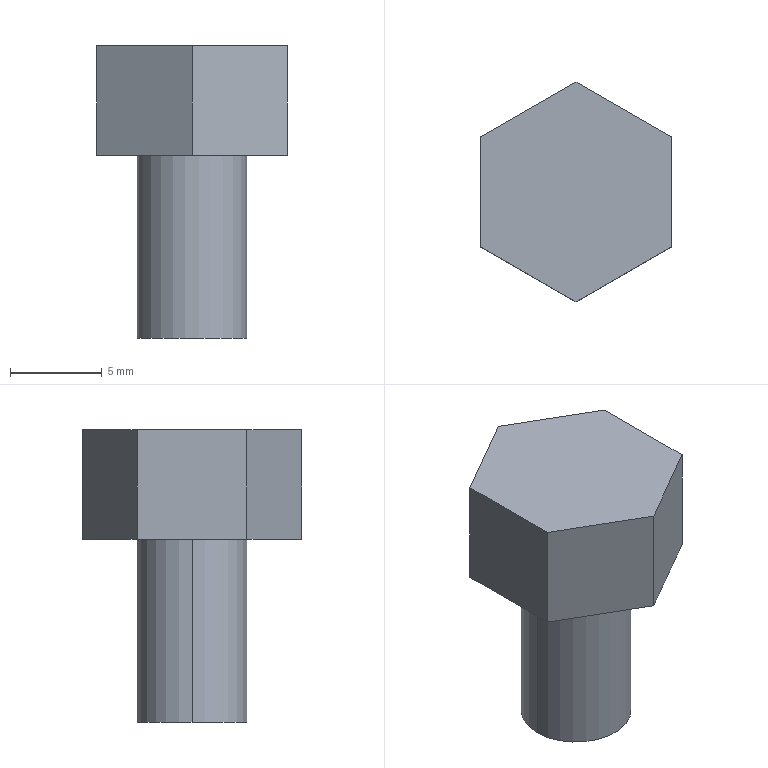Part | SolidWorks | features Extrusion 1, ICE 1 | 1 solid | 11 faces | box 10.392 x 12 x 16 mm | volume 843.928 mm3 | plane 9 | cylinder 2 | commonest cylinder face diameters 6 x2
STEP:
#1=CARTESIAN_POINT('',(3.,0.,10.));
#2=VERTEX_POINT('',#1);
#3=CARTESIAN_POINT('',(-3.,0.,10.));
#4=VERTEX_POINT('',#3);
#5=CARTESIAN_POINT('',(0.,0.,10.));
#6=DIRECTION('',(0.,0.,1.));
#7=DIRECTION('',(1.,0.,0.));
#8=AXIS2_PLACEMENT_3D('',#5,#6,#7);
#9=CIRCLE('',#8,3.);
#10=EDGE_CURVE('',#2,#4,#9,.T.);
#11=ORIENTED_EDGE('',*,*,#10,.F.);
#12=CARTESIAN_POINT('',(3.,0.,0.));
#13=VERTEX_POINT('',#12);
#14=CARTESIAN_POINT('',(3.,0.,10.));
#15=DIRECTION('',(0.,0.,-1.));
#16=VECTOR('',#15,1000.);
#17=LINE('',#14,#16);
#18=EDGE_CURVE('',#2,#13,#17,.T.);
#19=ORIENTED_EDGE('',*,*,#18,.T.);
#20=CARTESIAN_POINT('',(-3.,0.,0.));
#21=VERTEX_POINT('',#20);
#22=CARTESIAN_POINT('',(0.,0.,0.));
#23=DIRECTION('',(0.,0.,1.));
#24=DIRECTION('',(1.,0.,0.));
#25=AXIS2_PLACEMENT_3D('',#22,#23,#24);
#26=CIRCLE('',#25,3.);
#27=EDGE_CURVE('',#13,#21,#26,.T.);
#28=ORIENTED_EDGE('',*,*,#27,.T.);
#29=CARTESIAN_POINT('',(-3.,0.,10.));
#30=DIRECTION('',(0.,0.,-1.));
#31=VECTOR('',#30,1000.);
#32=LINE('',#29,#31);
#33=EDGE_CURVE('',#4,#21,#32,.T.);
#34=ORIENTED_EDGE('',*,*,#33,.F.);
#35=EDGE_LOOP('',(#11,#19,#28,#34));
#36=FACE_OUTER_BOUND('',#35,.T.);
#37=CARTESIAN_POINT('',(0.,0.,10.));
#38=DIRECTION('',(0.,0.,-1.));
#39=DIRECTION('',(-1.,0.,0.));
#40=AXIS2_PLACEMENT_3D('',#37,#38,#39);
#41=CYLINDRICAL_SURFACE('',#40,3.);
#42=ADVANCED_FACE('',(#36),#41,.T.);
#43=ORIENTED_EDGE('',*,*,#18,.F.);
#44=CARTESIAN_POINT('',(0.,0.,10.));
#45=DIRECTION('',(0.,0.,1.));
#46=DIRECTION('',(1.,0.,0.));
#47=AXIS2_PLACEMENT_3D('',#44,#45,#46);
#48=CIRCLE('',#47,3.);
#49=EDGE_CURVE('',#4,#2,#48,.T.);
#50=ORIENTED_EDGE('',*,*,#49,.F.);
#51=ORIENTED_EDGE('',*,*,#33,.T.);
#52=CARTESIAN_POINT('',(0.,0.,0.));
#53=DIRECTION('',(0.,0.,1.));
#54=DIRECTION('',(1.,0.,0.));
#55=AXIS2_PLACEMENT_3D('',#52,#53,#54);
#56=CIRCLE('',#55,3.);
#57=EDGE_CURVE('',#21,#13,#56,.T.);
#58=ORIENTED_EDGE('',*,*,#57,.T.);
#59=EDGE_LOOP('',(#43,#50,#51,#58));
#60=FACE_OUTER_BOUND('',#59,.T.);
#61=CARTESIAN_POINT('',(0.,0.,10.));
#62=DIRECTION('',(0.,0.,-1.));
#63=DIRECTION('',(-1.,0.,0.));
#64=AXIS2_PLACEMENT_3D('',#61,#62,#63);
#65=CYLINDRICAL_SURFACE('',#64,3.);
#66=ADVANCED_FACE('',(#60),#65,.T.);
#67=ORIENTED_EDGE('',*,*,#57,.F.);
#68=ORIENTED_EDGE('',*,*,#27,.F.);
#69=EDGE_LOOP('',(#67,#68));
#70=FACE_OUTER_BOUND('',#69,.T.);
#71=CARTESIAN_POINT('',(0.,0.,0.));
#72=DIRECTION('',(0.,0.,1.));
#73=DIRECTION('',(1.,0.,0.));
#74=AXIS2_PLACEMENT_3D('',#71,#72,#73);
#75=PLANE('',#74);
#76=ADVANCED_FACE('',(#70),#75,.F.);
#77=CARTESIAN_POINT('',(-5.196,3.,10.));
#78=VERTEX_POINT('',#77);
#79=CARTESIAN_POINT('',(-5.196,-3.,10.));
#80=VERTEX_POINT('',#79);
#81=CARTESIAN_POINT('',(-5.196,3.,10.));
#82=DIRECTION('',(0.,-1.,0.));
#83=VECTOR('',#82,1000.);
#84=LINE('',#81,#83);
#85=EDGE_CURVE('',#78,#80,#84,.T.);
#86=ORIENTED_EDGE('',*,*,#85,.T.);
#87=CARTESIAN_POINT('',(-5.196,-3.,16.));
#88=VERTEX_POINT('',#87);
#89=CARTESIAN_POINT('',(-5.196,-3.,16.));
#90=DIRECTION('',(0.,0.,-1.));
#91=VECTOR('',#90,1000.);
#92=LINE('',#89,#91);
#93=EDGE_CURVE('',#88,#80,#92,.T.);
#94=ORIENTED_EDGE('',*,*,#93,.F.);
#95=CARTESIAN_POINT('',(-5.196,3.,16.));
#96=VERTEX_POINT('',#95);
#97=CARTESIAN_POINT('',(-5.196,3.,16.));
#98=DIRECTION('',(0.,-1.,0.));
#99=VECTOR('',#98,1000.);
#100=LINE('',#97,#99);
#101=EDGE_CURVE('',#96,#88,#100,.T.);
#102=ORIENTED_EDGE('',*,*,#101,.F.);
#103=CARTESIAN_POINT('',(-5.196,3.,16.));
#104=DIRECTION('',(0.,0.,-1.));
#105=VECTOR('',#104,1000.);
#106=LINE('',#103,#105);
#107=EDGE_CURVE('',#96,#78,#106,.T.);
#108=ORIENTED_EDGE('',*,*,#107,.T.);
#109=EDGE_LOOP('',(#86,#94,#102,#108));
#110=FACE_OUTER_BOUND('',#109,.T.);
#111=CARTESIAN_POINT('',(-5.196,3.,16.));
#112=DIRECTION('',(1.,0.,0.));
#113=DIRECTION('',(0.,0.,-1.));
#114=AXIS2_PLACEMENT_3D('',#111,#112,#113);
#115=PLANE('',#114);
#116=ADVANCED_FACE('',(#110),#115,.F.);
#117=CARTESIAN_POINT('',(0.,-6.,10.));
#118=VERTEX_POINT('',#117);
#119=CARTESIAN_POINT('',(-5.196,-3.,10.));
#120=DIRECTION('',(0.866,-0.5,0.));
#121=VECTOR('',#120,1000.);
#122=LINE('',#119,#121);
#123=EDGE_CURVE('',#80,#118,#122,.T.);
#124=ORIENTED_EDGE('',*,*,#123,.T.);
#125=CARTESIAN_POINT('',(0.,-6.,16.));
#126=VERTEX_POINT('',#125);
#127=CARTESIAN_POINT('',(0.,-6.,16.));
#128=DIRECTION('',(0.,0.,-1.));
#129=VECTOR('',#128,1000.);
#130=LINE('',#127,#129);
#131=EDGE_CURVE('',#126,#118,#130,.T.);
#132=ORIENTED_EDGE('',*,*,#131,.F.);
#133=CARTESIAN_POINT('',(-5.196,-3.,16.));
#134=DIRECTION('',(0.866,-0.5,0.));
#135=VECTOR('',#134,1000.);
#136=LINE('',#133,#135);
#137=EDGE_CURVE('',#88,#126,#136,.T.);
#138=ORIENTED_EDGE('',*,*,#137,.F.);
#139=ORIENTED_EDGE('',*,*,#93,.T.);
#140=EDGE_LOOP('',(#124,#132,#138,#139));
#141=FACE_OUTER_BOUND('',#140,.T.);
#142=CARTESIAN_POINT('',(-5.196,-3.,16.));
#143=DIRECTION('',(0.5,0.866,0.));
#144=DIRECTION('',(-0.866,0.5,0.));
#145=AXIS2_PLACEMENT_3D('',#142,#143,#144);
#146=PLANE('',#145);
#147=ADVANCED_FACE('',(#141),#146,.F.);
#148=CARTESIAN_POINT('',(5.196,-3.,10.));
#149=VERTEX_POINT('',#148);
#150=CARTESIAN_POINT('',(0.,-6.,10.));
#151=DIRECTION('',(0.866,0.5,0.));
#152=VECTOR('',#151,1000.);
#153=LINE('',#150,#152);
#154=EDGE_CURVE('',#118,#149,#153,.T.);
#155=ORIENTED_EDGE('',*,*,#154,.T.);
#156=CARTESIAN_POINT('',(5.196,-3.,16.));
#157=VERTEX_POINT('',#156);
#158=CARTESIAN_POINT('',(5.196,-3.,16.));
#159=DIRECTION('',(0.,0.,-1.));
#160=VECTOR('',#159,1000.);
#161=LINE('',#158,#160);
#162=EDGE_CURVE('',#157,#149,#161,.T.);
#163=ORIENTED_EDGE('',*,*,#162,.F.);
#164=CARTESIAN_POINT('',(0.,-6.,16.));
#165=DIRECTION('',(0.866,0.5,0.));
#166=VECTOR('',#165,1000.);
#167=LINE('',#164,#166);
#168=EDGE_CURVE('',#126,#157,#167,.T.);
#169=ORIENTED_EDGE('',*,*,#168,.F.);
#170=ORIENTED_EDGE('',*,*,#131,.T.);
#171=EDGE_LOOP('',(#155,#163,#169,#170));
#172=FACE_OUTER_BOUND('',#171,.T.);
#173=CARTESIAN_POINT('',(0.,-6.,16.));
#174=DIRECTION('',(-0.5,0.866,0.));
#175=DIRECTION('',(-0.866,-0.5,0.));
#176=AXIS2_PLACEMENT_3D('',#173,#174,#175);
#177=PLANE('',#176);
#178=ADVANCED_FACE('',(#172),#177,.F.);
#179=CARTESIAN_POINT('',(5.196,3.,10.));
#180=VERTEX_POINT('',#179);
#181=CARTESIAN_POINT('',(5.196,-3.,10.));
#182=DIRECTION('',(0.,1.,0.));
#183=VECTOR('',#182,1000.);
#184=LINE('',#181,#183);
#185=EDGE_CURVE('',#149,#180,#184,.T.);
#186=ORIENTED_EDGE('',*,*,#185,.T.);
#187=CARTESIAN_POINT('',(5.196,3.,16.));
#188=VERTEX_POINT('',#187);
#189=CARTESIAN_POINT('',(5.196,3.,16.));
#190=DIRECTION('',(0.,0.,-1.));
#191=VECTOR('',#190,1000.);
#192=LINE('',#189,#191);
#193=EDGE_CURVE('',#188,#180,#192,.T.);
#194=ORIENTED_EDGE('',*,*,#193,.F.);
#195=CARTESIAN_POINT('',(5.196,-3.,16.));
#196=DIRECTION('',(0.,1.,0.));
#197=VECTOR('',#196,1000.);
#198=LINE('',#195,#197);
#199=EDGE_CURVE('',#157,#188,#198,.T.);
#200=ORIENTED_EDGE('',*,*,#199,.F.);
#201=ORIENTED_EDGE('',*,*,#162,.T.);
#202=EDGE_LOOP('',(#186,#194,#200,#201));
#203=FACE_OUTER_BOUND('',#202,.T.);
#204=CARTESIAN_POINT('',(5.196,-3.,16.));
#205=DIRECTION('',(-1.,0.,0.));
#206=DIRECTION('',(0.,-1.,0.));
#207=AXIS2_PLACEMENT_3D('',#204,#205,#206);
#208=PLANE('',#207);
#209=ADVANCED_FACE('',(#203),#208,.F.);
#210=CARTESIAN_POINT('',(0.,6.,10.));
#211=VERTEX_POINT('',#210);
#212=CARTESIAN_POINT('',(5.196,3.,10.));
#213=DIRECTION('',(-0.866,0.5,0.));
#214=VECTOR('',#213,1000.);
#215=LINE('',#212,#214);
#216=EDGE_CURVE('',#180,#211,#215,.T.);
#217=ORIENTED_EDGE('',*,*,#216,.T.);
#218=CARTESIAN_POINT('',(0.,6.,16.));
#219=VERTEX_POINT('',#218);
#220=CARTESIAN_POINT('',(0.,6.,16.));
#221=DIRECTION('',(0.,0.,-1.));
#222=VECTOR('',#221,1000.);
#223=LINE('',#220,#222);
#224=EDGE_CURVE('',#219,#211,#223,.T.);
#225=ORIENTED_EDGE('',*,*,#224,.F.);
#226=CARTESIAN_POINT('',(5.196,3.,16.));
#227=DIRECTION('',(-0.866,0.5,0.));
#228=VECTOR('',#227,1000.);
#229=LINE('',#226,#228);
#230=EDGE_CURVE('',#188,#219,#229,.T.);
#231=ORIENTED_EDGE('',*,*,#230,.F.);
#232=ORIENTED_EDGE('',*,*,#193,.T.);
#233=EDGE_LOOP('',(#217,#225,#231,#232));
#234=FACE_OUTER_BOUND('',#233,.T.);
#235=CARTESIAN_POINT('',(5.196,3.,16.));
#236=DIRECTION('',(-0.5,-0.866,0.));
#237=DIRECTION('',(0.866,-0.5,0.));
#238=AXIS2_PLACEMENT_3D('',#235,#236,#237);
#239=PLANE('',#238);
#240=ADVANCED_FACE('',(#234),#239,.F.);
#241=CARTESIAN_POINT('',(0.,6.,10.));
#242=DIRECTION('',(-0.866,-0.5,0.));
#243=VECTOR('',#242,1000.);
#244=LINE('',#241,#243);
#245=EDGE_CURVE('',#211,#78,#244,.T.);
#246=ORIENTED_EDGE('',*,*,#245,.T.);
#247=ORIENTED_EDGE('',*,*,#107,.F.);
#248=CARTESIAN_POINT('',(0.,6.,16.));
#249=DIRECTION('',(-0.866,-0.5,0.));
#250=VECTOR('',#249,1000.);
#251=LINE('',#248,#250);
#252=EDGE_CURVE('',#219,#96,#251,.T.);
#253=ORIENTED_EDGE('',*,*,#252,.F.);
#254=ORIENTED_EDGE('',*,*,#224,.T.);
#255=EDGE_LOOP('',(#246,#247,#253,#254));
#256=FACE_OUTER_BOUND('',#255,.T.);
#257=CARTESIAN_POINT('',(0.,6.,16.));
#258=DIRECTION('',(0.5,-0.866,0.));
#259=DIRECTION('',(0.866,0.5,0.));
#260=AXIS2_PLACEMENT_3D('',#257,#258,#259);
#261=PLANE('',#260);
#262=ADVANCED_FACE('',(#256),#261,.F.);
#263=ORIENTED_EDGE('',*,*,#101,.T.);
#264=ORIENTED_EDGE('',*,*,#137,.T.);
#265=ORIENTED_EDGE('',*,*,#168,.T.);
#266=ORIENTED_EDGE('',*,*,#199,.T.);
#267=ORIENTED_EDGE('',*,*,#230,.T.);
#268=ORIENTED_EDGE('',*,*,#252,.T.);
#269=EDGE_LOOP('',(#263,#264,#265,#266,#267,#268));
#270=FACE_OUTER_BOUND('',#269,.T.);
#271=CARTESIAN_POINT('',(0.,0.,16.));
#272=DIRECTION('',(0.,0.,1.));
#273=DIRECTION('',(1.,0.,0.));
#274=AXIS2_PLACEMENT_3D('',#271,#272,#273);
#275=PLANE('',#274);
#276=ADVANCED_FACE('',(#270),#275,.T.);
#277=ORIENTED_EDGE('',*,*,#49,.T.);
#278=ORIENTED_EDGE('',*,*,#10,.T.);
#279=EDGE_LOOP('',(#277,#278));
#280=FACE_BOUND('',#279,.T.);
#281=ORIENTED_EDGE('',*,*,#85,.F.);
#282=ORIENTED_EDGE('',*,*,#245,.F.);
#283=ORIENTED_EDGE('',*,*,#216,.F.);
#284=ORIENTED_EDGE('',*,*,#185,.F.);
#285=ORIENTED_EDGE('',*,*,#154,.F.);
#286=ORIENTED_EDGE('',*,*,#123,.F.);
#287=EDGE_LOOP('',(#281,#282,#283,#284,#285,#286));
#288=FACE_OUTER_BOUND('',#287,.T.);
#289=CARTESIAN_POINT('',(0.,0.,10.));
#290=DIRECTION('',(0.,0.,1.));
#291=DIRECTION('',(1.,0.,0.));
#292=AXIS2_PLACEMENT_3D('',#289,#290,#291);
#293=PLANE('',#292);
#294=ADVANCED_FACE('',(#280,#288),#293,.F.);
#295=CLOSED_SHELL('',(#42,#66,#76,#116,#147,#178,#209,#240,#262,#276,#294));
#296=MANIFOLD_SOLID_BREP('',#295);
#297=CARTESIAN_POINT('',(0.,0.,0.));
#298=DIRECTION('',(0.,0.,1.));
#299=DIRECTION('',(1.,0.,0.));
#300=AXIS2_PLACEMENT_3D('',#297,#298,#299);
#301=(LENGTH_UNIT()NAMED_UNIT(*)SI_UNIT(.MILLI.,.METRE.));
#302=UNCERTAINTY_MEASURE_WITH_UNIT(LENGTH_MEASURE(0.00001),#301,'','');
#303=(NAMED_UNIT(*)PLANE_ANGLE_UNIT()SI_UNIT($,.RADIAN.));
#304=(NAMED_UNIT(*)SI_UNIT($,.STERADIAN.)SOLID_ANGLE_UNIT());
#305=(GEOMETRIC_REPRESENTATION_CONTEXT(3)GLOBAL_UNCERTAINTY_ASSIGNED_CONTEXT((#302))GLOBAL_UNIT_ASSIGNED_CONTEXT((#301,#303,#304))REPRESENTATION_CONTEXT('',''));
#306=ADVANCED_BREP_SHAPE_REPRESENTATION('',(#296,#300),#305);